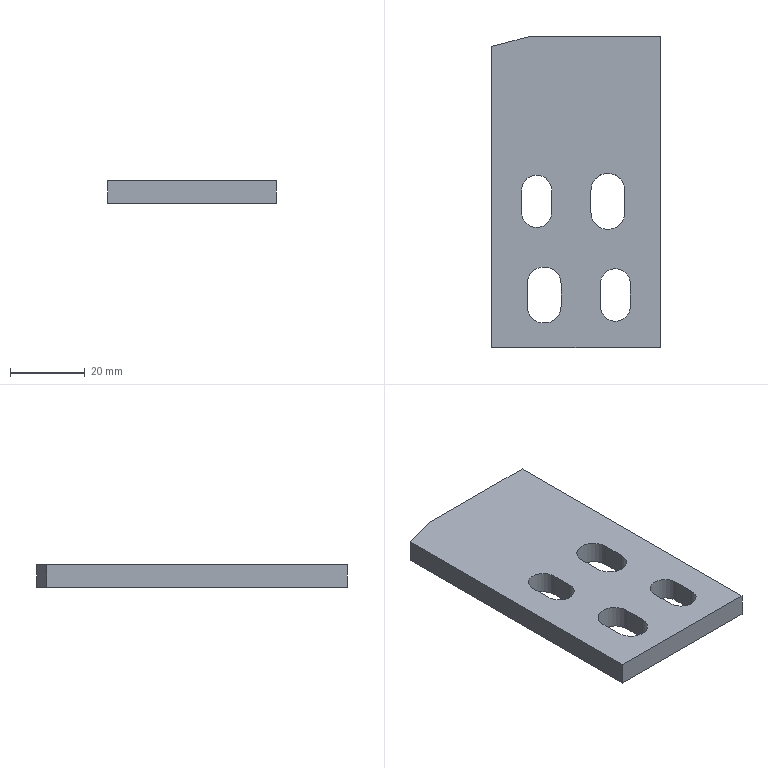Part | STEP file | gslz 2016.10.28-13_id1726_x_t | 1 solid | 23 faces | box 45 x 83 x 6 mm | volume 19739 mm3 | plane 15 | cylinder 8 | commonest cylinder face diameters 8 x4 9 x4